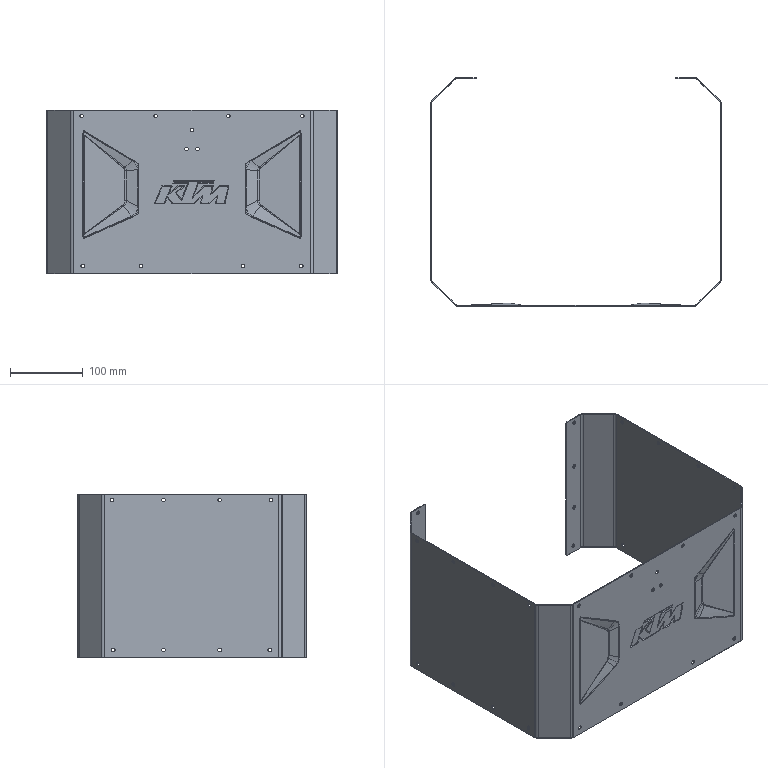Part | SolidWorks | features BaseBody 1 | 1 solid | 230 faces | box 399.8 x 313.601 x 224 mm | volume 283664 mm3 | cylinder 120 | spline 57 | plane 53 | commonest cylinder face diameters 5.2 x40 1.189 x30 4.9 x18 5 x12 10 x8 12.4 x8